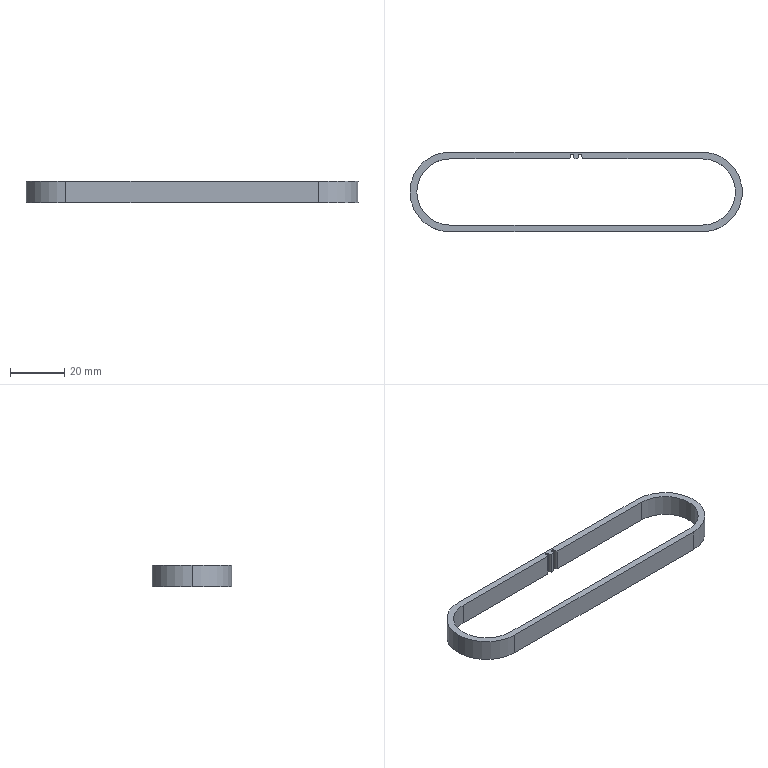Part | STEP file | Timing belt 270-3M-8mm wide_28-28 teeth H93 | 1 solid | 30 faces | box 122.34 x 29.34 x 8 mm | volume 5374 mm3 | cylinder 20 | plane 10 | commonest cylinder face diameters 0.6 x6 3.9 x6 24.34 x3 29.34 x3 0.2 x2